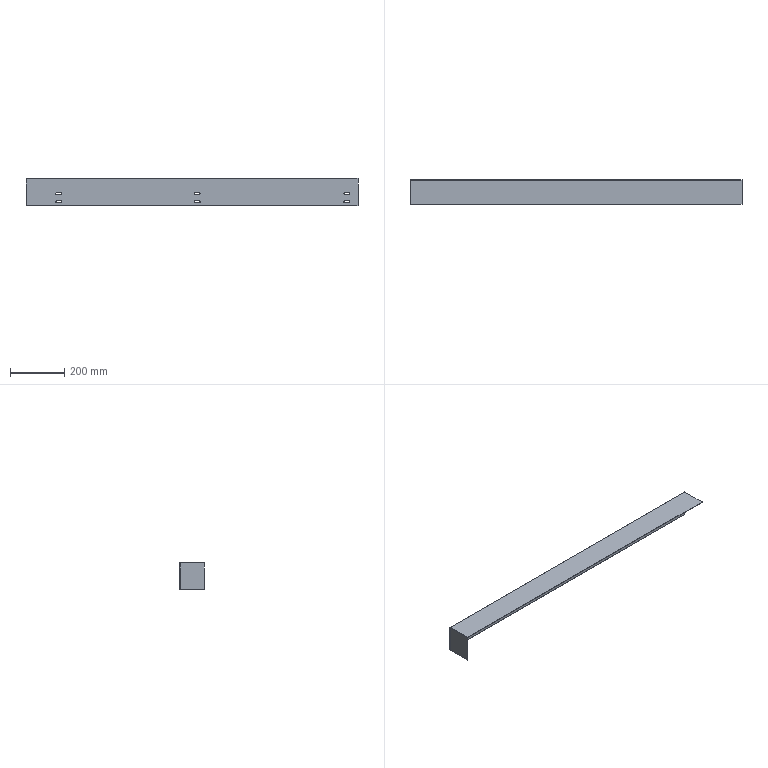Part | SolidWorks | features BaseBody 1 | 1 solid | 41 faces | box 1222 x 91.5 x 101.5 mm | volume 361742 mm3 | plane 25 | cylinder 16 | commonest cylinder face diameters 6 x12 1.473 x2 4.473 x2
STEP:
#1=CARTESIAN_POINT('',(561.,0.,48.));
#2=VERTEX_POINT('',#1);
#3=CARTESIAN_POINT('',(561.,1.5,48.));
#4=VERTEX_POINT('',#3);
#5=CARTESIAN_POINT('',(561.,-90.001,48.));
#6=DIRECTION('',(0.,1.,0.));
#7=VECTOR('',#6,1000.);
#8=LINE('',#5,#7);
#9=EDGE_CURVE('',#2,#4,#8,.T.);
#10=ORIENTED_EDGE('',*,*,#9,.T.);
#11=CARTESIAN_POINT('',(576.,1.5,48.));
#12=VERTEX_POINT('',#11);
#13=CARTESIAN_POINT('',(561.,1.5,48.));
#14=DIRECTION('',(1.,0.,0.));
#15=VECTOR('',#14,1000.);
#16=LINE('',#13,#15);
#17=EDGE_CURVE('',#4,#12,#16,.T.);
#18=ORIENTED_EDGE('',*,*,#17,.T.);
#19=CARTESIAN_POINT('',(576.,0.,48.));
#20=VERTEX_POINT('',#19);
#21=CARTESIAN_POINT('',(576.,-90.001,48.));
#22=DIRECTION('',(0.,1.,0.));
#23=VECTOR('',#22,1000.);
#24=LINE('',#21,#23);
#25=EDGE_CURVE('',#20,#12,#24,.T.);
#26=ORIENTED_EDGE('',*,*,#25,.F.);
#27=CARTESIAN_POINT('',(561.,0.,48.));
#28=DIRECTION('',(1.,0.,0.));
#29=VECTOR('',#28,1000.);
#30=LINE('',#27,#29);
#31=EDGE_CURVE('',#2,#20,#30,.T.);
#32=ORIENTED_EDGE('',*,*,#31,.F.);
#33=EDGE_LOOP('',(#10,#18,#26,#32));
#34=FACE_OUTER_BOUND('',#33,.T.);
#35=CARTESIAN_POINT('',(561.,-90.001,48.));
#36=DIRECTION('',(0.,0.,1.));
#37=DIRECTION('',(0.,-1.,0.));
#38=AXIS2_PLACEMENT_3D('',#35,#36,#37);
#39=PLANE('',#38);
#40=ADVANCED_FACE('',(#34),#39,.F.);
#41=ORIENTED_EDGE('',*,*,#25,.T.);
#42=CARTESIAN_POINT('',(576.,1.5,42.));
#43=VERTEX_POINT('',#42);
#44=CARTESIAN_POINT('',(576.,1.5,45.));
#45=DIRECTION('',(0.,1.,0.));
#46=DIRECTION('',(0.,0.,1.));
#47=AXIS2_PLACEMENT_3D('',#44,#45,#46);
#48=CIRCLE('',#47,3.);
#49=EDGE_CURVE('',#12,#43,#48,.T.);
#50=ORIENTED_EDGE('',*,*,#49,.T.);
#51=CARTESIAN_POINT('',(576.,0.,42.));
#52=VERTEX_POINT('',#51);
#53=CARTESIAN_POINT('',(576.,-90.001,42.));
#54=DIRECTION('',(0.,1.,0.));
#55=VECTOR('',#54,1000.);
#56=LINE('',#53,#55);
#57=EDGE_CURVE('',#52,#43,#56,.T.);
#58=ORIENTED_EDGE('',*,*,#57,.F.);
#59=CARTESIAN_POINT('',(576.,0.,45.));
#60=DIRECTION('',(0.,1.,0.));
#61=DIRECTION('',(0.,0.,-1.));
#62=AXIS2_PLACEMENT_3D('',#59,#60,#61);
#63=CIRCLE('',#62,3.);
#64=EDGE_CURVE('',#20,#52,#63,.T.);
#65=ORIENTED_EDGE('',*,*,#64,.F.);
#66=EDGE_LOOP('',(#41,#50,#58,#65));
#67=FACE_OUTER_BOUND('',#66,.T.);
#68=CARTESIAN_POINT('',(576.,-90.001,45.));
#69=DIRECTION('',(0.,1.,0.));
#70=DIRECTION('',(0.,0.,1.));
#71=AXIS2_PLACEMENT_3D('',#68,#69,#70);
#72=CYLINDRICAL_SURFACE('',#71,3.);
#73=ADVANCED_FACE('',(#67),#72,.F.);
#74=ORIENTED_EDGE('',*,*,#57,.T.);
#75=CARTESIAN_POINT('',(561.,1.5,42.));
#76=VERTEX_POINT('',#75);
#77=CARTESIAN_POINT('',(561.,1.5,42.));
#78=DIRECTION('',(-1.,0.,0.));
#79=VECTOR('',#78,1000.);
#80=LINE('',#77,#79);
#81=EDGE_CURVE('',#43,#76,#80,.T.);
#82=ORIENTED_EDGE('',*,*,#81,.T.);
#83=CARTESIAN_POINT('',(561.,0.,42.));
#84=VERTEX_POINT('',#83);
#85=CARTESIAN_POINT('',(561.,-90.001,42.));
#86=DIRECTION('',(0.,1.,0.));
#87=VECTOR('',#86,1000.);
#88=LINE('',#85,#87);
#89=EDGE_CURVE('',#84,#76,#88,.T.);
#90=ORIENTED_EDGE('',*,*,#89,.F.);
#91=CARTESIAN_POINT('',(561.,0.,42.));
#92=DIRECTION('',(-1.,0.,0.));
#93=VECTOR('',#92,1000.);
#94=LINE('',#91,#93);
#95=EDGE_CURVE('',#52,#84,#94,.T.);
#96=ORIENTED_EDGE('',*,*,#95,.F.);
#97=EDGE_LOOP('',(#74,#82,#90,#96));
#98=FACE_OUTER_BOUND('',#97,.T.);
#99=CARTESIAN_POINT('',(561.,-90.001,42.));
#100=DIRECTION('',(0.,0.,-1.));
#101=DIRECTION('',(-1.,0.,0.));
#102=AXIS2_PLACEMENT_3D('',#99,#100,#101);
#103=PLANE('',#102);
#104=ADVANCED_FACE('',(#98),#103,.F.);
#105=ORIENTED_EDGE('',*,*,#89,.T.);
#106=CARTESIAN_POINT('',(561.,1.5,45.));
#107=DIRECTION('',(0.,1.,0.));
#108=DIRECTION('',(0.,0.,1.));
#109=AXIS2_PLACEMENT_3D('',#106,#107,#108);
#110=CIRCLE('',#109,3.);
#111=EDGE_CURVE('',#76,#4,#110,.T.);
#112=ORIENTED_EDGE('',*,*,#111,.T.);
#113=ORIENTED_EDGE('',*,*,#9,.F.);
#114=CARTESIAN_POINT('',(561.,0.,45.));
#115=DIRECTION('',(0.,1.,0.));
#116=DIRECTION('',(0.,0.,-1.));
#117=AXIS2_PLACEMENT_3D('',#114,#115,#116);
#118=CIRCLE('',#117,3.);
#119=EDGE_CURVE('',#84,#2,#118,.T.);
#120=ORIENTED_EDGE('',*,*,#119,.F.);
#121=EDGE_LOOP('',(#105,#112,#113,#120));
#122=FACE_OUTER_BOUND('',#121,.T.);
#123=CARTESIAN_POINT('',(561.,-90.001,45.));
#124=DIRECTION('',(0.,1.,0.));
#125=DIRECTION('',(0.,0.,1.));
#126=AXIS2_PLACEMENT_3D('',#123,#124,#125);
#127=CYLINDRICAL_SURFACE('',#126,3.);
#128=ADVANCED_FACE('',(#122),#127,.F.);
#129=CARTESIAN_POINT('',(561.,0.,18.));
#130=VERTEX_POINT('',#129);
#131=CARTESIAN_POINT('',(561.,1.5,18.));
#132=VERTEX_POINT('',#131);
#133=CARTESIAN_POINT('',(561.,-90.001,18.));
#134=DIRECTION('',(0.,1.,0.));
#135=VECTOR('',#134,1000.);
#136=LINE('',#133,#135);
#137=EDGE_CURVE('',#130,#132,#136,.T.);
#138=ORIENTED_EDGE('',*,*,#137,.T.);
#139=CARTESIAN_POINT('',(576.,1.5,18.));
#140=VERTEX_POINT('',#139);
#141=CARTESIAN_POINT('',(561.,1.5,18.));
#142=DIRECTION('',(1.,0.,0.));
#143=VECTOR('',#142,1000.);
#144=LINE('',#141,#143);
#145=EDGE_CURVE('',#132,#140,#144,.T.);
#146=ORIENTED_EDGE('',*,*,#145,.T.);
#147=CARTESIAN_POINT('',(576.,0.,18.));
#148=VERTEX_POINT('',#147);
#149=CARTESIAN_POINT('',(576.,-90.001,18.));
#150=DIRECTION('',(0.,1.,0.));
#151=VECTOR('',#150,1000.);
#152=LINE('',#149,#151);
#153=EDGE_CURVE('',#148,#140,#152,.T.);
#154=ORIENTED_EDGE('',*,*,#153,.F.);
#155=CARTESIAN_POINT('',(561.,0.,18.));
#156=DIRECTION('',(1.,0.,0.));
#157=VECTOR('',#156,1000.);
#158=LINE('',#155,#157);
#159=EDGE_CURVE('',#130,#148,#158,.T.);
#160=ORIENTED_EDGE('',*,*,#159,.F.);
#161=EDGE_LOOP('',(#138,#146,#154,#160));
#162=FACE_OUTER_BOUND('',#161,.T.);
#163=CARTESIAN_POINT('',(561.,-90.001,18.));
#164=DIRECTION('',(0.,0.,1.));
#165=DIRECTION('',(0.,-1.,0.));
#166=AXIS2_PLACEMENT_3D('',#163,#164,#165);
#167=PLANE('',#166);
#168=ADVANCED_FACE('',(#162),#167,.F.);
#169=ORIENTED_EDGE('',*,*,#153,.T.);
#170=CARTESIAN_POINT('',(576.,1.5,12.));
#171=VERTEX_POINT('',#170);
#172=CARTESIAN_POINT('',(576.,1.5,15.));
#173=DIRECTION('',(0.,1.,0.));
#174=DIRECTION('',(0.,0.,1.));
#175=AXIS2_PLACEMENT_3D('',#172,#173,#174);
#176=CIRCLE('',#175,3.);
#177=EDGE_CURVE('',#140,#171,#176,.T.);
#178=ORIENTED_EDGE('',*,*,#177,.T.);
#179=CARTESIAN_POINT('',(576.,0.,12.));
#180=VERTEX_POINT('',#179);
#181=CARTESIAN_POINT('',(576.,-90.001,12.));
#182=DIRECTION('',(0.,1.,0.));
#183=VECTOR('',#182,1000.);
#184=LINE('',#181,#183);
#185=EDGE_CURVE('',#180,#171,#184,.T.);
#186=ORIENTED_EDGE('',*,*,#185,.F.);
#187=CARTESIAN_POINT('',(576.,0.,15.));
#188=DIRECTION('',(0.,1.,0.));
#189=DIRECTION('',(0.,0.,-1.));
#190=AXIS2_PLACEMENT_3D('',#187,#188,#189);
#191=CIRCLE('',#190,3.);
#192=EDGE_CURVE('',#148,#180,#191,.T.);
#193=ORIENTED_EDGE('',*,*,#192,.F.);
#194=EDGE_LOOP('',(#169,#178,#186,#193));
#195=FACE_OUTER_BOUND('',#194,.T.);
#196=CARTESIAN_POINT('',(576.,-90.001,15.));
#197=DIRECTION('',(0.,1.,0.));
#198=DIRECTION('',(0.,0.,1.));
#199=AXIS2_PLACEMENT_3D('',#196,#197,#198);
#200=CYLINDRICAL_SURFACE('',#199,3.);
#201=ADVANCED_FACE('',(#195),#200,.F.);
#202=ORIENTED_EDGE('',*,*,#185,.T.);
#203=CARTESIAN_POINT('',(561.,1.5,12.));
#204=VERTEX_POINT('',#203);
#205=CARTESIAN_POINT('',(561.,1.5,12.));
#206=DIRECTION('',(-1.,0.,0.));
#207=VECTOR('',#206,1000.);
#208=LINE('',#205,#207);
#209=EDGE_CURVE('',#171,#204,#208,.T.);
#210=ORIENTED_EDGE('',*,*,#209,.T.);
#211=CARTESIAN_POINT('',(561.,0.,12.));
#212=VERTEX_POINT('',#211);
#213=CARTESIAN_POINT('',(561.,-90.001,12.));
#214=DIRECTION('',(0.,1.,0.));
#215=VECTOR('',#214,1000.);
#216=LINE('',#213,#215);
#217=EDGE_CURVE('',#212,#204,#216,.T.);
#218=ORIENTED_EDGE('',*,*,#217,.F.);
#219=CARTESIAN_POINT('',(561.,0.,12.));
#220=DIRECTION('',(-1.,0.,0.));
#221=VECTOR('',#220,1000.);
#222=LINE('',#219,#221);
#223=EDGE_CURVE('',#180,#212,#222,.T.);
#224=ORIENTED_EDGE('',*,*,#223,.F.);
#225=EDGE_LOOP('',(#202,#210,#218,#224));
#226=FACE_OUTER_BOUND('',#225,.T.);
#227=CARTESIAN_POINT('',(561.,-90.001,12.));
#228=DIRECTION('',(0.,0.,-1.));
#229=DIRECTION('',(-1.,0.,0.));
#230=AXIS2_PLACEMENT_3D('',#227,#228,#229);
#231=PLANE('',#230);
#232=ADVANCED_FACE('',(#226),#231,.F.);
#233=ORIENTED_EDGE('',*,*,#217,.T.);
#234=CARTESIAN_POINT('',(561.,1.5,15.));
#235=DIRECTION('',(0.,1.,0.));
#236=DIRECTION('',(0.,0.,1.));
#237=AXIS2_PLACEMENT_3D('',#234,#235,#236);
#238=CIRCLE('',#237,3.);
#239=EDGE_CURVE('',#204,#132,#238,.T.);
#240=ORIENTED_EDGE('',*,*,#239,.T.);
#241=ORIENTED_EDGE('',*,*,#137,.F.);
#242=CARTESIAN_POINT('',(561.,0.,15.));
#243=DIRECTION('',(0.,1.,0.));
#244=DIRECTION('',(0.,0.,-1.));
#245=AXIS2_PLACEMENT_3D('',#242,#243,#244);
#246=CIRCLE('',#245,3.);
#247=EDGE_CURVE('',#212,#130,#246,.T.);
#248=ORIENTED_EDGE('',*,*,#247,.F.);
#249=EDGE_LOOP('',(#233,#240,#241,#248));
#250=FACE_OUTER_BOUND('',#249,.T.);
#251=CARTESIAN_POINT('',(561.,-90.001,15.));
#252=DIRECTION('',(0.,1.,0.));
#253=DIRECTION('',(0.,0.,1.));
#254=AXIS2_PLACEMENT_3D('',#251,#252,#253);
#255=CYLINDRICAL_SURFACE('',#254,3.);
#256=ADVANCED_FACE('',(#250),#255,.F.);
#257=CARTESIAN_POINT('',(26.,0.,12.));
#258=VERTEX_POINT('',#257);
#259=CARTESIAN_POINT('',(26.,1.5,12.));
#260=VERTEX_POINT('',#259);
#261=CARTESIAN_POINT('',(26.,-90.001,12.));
#262=DIRECTION('',(0.,1.,0.));
#263=VECTOR('',#262,1000.);
#264=LINE('',#261,#263);
#265=EDGE_CURVE('',#258,#260,#264,.T.);
#266=ORIENTED_EDGE('',*,*,#265,.T.);
#267=CARTESIAN_POINT('',(11.,1.5,12.));
#268=VERTEX_POINT('',#267);
#269=CARTESIAN_POINT('',(26.,1.5,12.));
#270=DIRECTION('',(-1.,0.,0.));
#271=VECTOR('',#270,1000.);
#272=LINE('',#269,#271);
#273=EDGE_CURVE('',#260,#268,#272,.T.);
#274=ORIENTED_EDGE('',*,*,#273,.T.);
#275=CARTESIAN_POINT('',(11.,0.,12.));
#276=VERTEX_POINT('',#275);
#277=CARTESIAN_POINT('',(11.,-90.001,12.));
#278=DIRECTION('',(0.,1.,0.));
#279=VECTOR('',#278,1000.);
#280=LINE('',#277,#279);
#281=EDGE_CURVE('',#276,#268,#280,.T.);
#282=ORIENTED_EDGE('',*,*,#281,.F.);
#283=CARTESIAN_POINT('',(26.,0.,12.));
#284=DIRECTION('',(-1.,0.,0.));
#285=VECTOR('',#284,1000.);
#286=LINE('',#283,#285);
#287=EDGE_CURVE('',#258,#276,#286,.T.);
#288=ORIENTED_EDGE('',*,*,#287,.F.);
#289=EDGE_LOOP('',(#266,#274,#282,#288));
#290=FACE_OUTER_BOUND('',#289,.T.);
#291=CARTESIAN_POINT('',(26.,-90.001,12.));
#292=DIRECTION('',(0.,0.,-1.));
#293=DIRECTION('',(-1.,0.,0.));
#294=AXIS2_PLACEMENT_3D('',#291,#292,#293);
#295=PLANE('',#294);
#296=ADVANCED_FACE('',(#290),#295,.F.);
#297=ORIENTED_EDGE('',*,*,#281,.T.);
#298=CARTESIAN_POINT('',(11.,1.5,18.));
#299=VERTEX_POINT('',#298);
#300=CARTESIAN_POINT('',(11.,1.5,15.));
#301=DIRECTION('',(0.,1.,0.));
#302=DIRECTION('',(0.,0.,-1.));
#303=AXIS2_PLACEMENT_3D('',#300,#301,#302);
#304=CIRCLE('',#303,3.);
#305=EDGE_CURVE('',#268,#299,#304,.T.);
#306=ORIENTED_EDGE('',*,*,#305,.T.);
#307=CARTESIAN_POINT('',(11.,0.,18.));
#308=VERTEX_POINT('',#307);
#309=CARTESIAN_POINT('',(11.,-90.001,18.));
#310=DIRECTION('',(0.,1.,0.));
#311=VECTOR('',#310,1000.);
#312=LINE('',#309,#311);
#313=EDGE_CURVE('',#308,#299,#312,.T.);
#314=ORIENTED_EDGE('',*,*,#313,.F.);
#315=CARTESIAN_POINT('',(11.,0.,15.));
#316=DIRECTION('',(0.,1.,0.));
#317=DIRECTION('',(0.,0.,-1.));
#318=AXIS2_PLACEMENT_3D('',#315,#316,#317);
#319=CIRCLE('',#318,3.);
#320=EDGE_CURVE('',#276,#308,#319,.T.);
#321=ORIENTED_EDGE('',*,*,#320,.F.);
#322=EDGE_LOOP('',(#297,#306,#314,#321));
#323=FACE_OUTER_BOUND('',#322,.T.);
#324=CARTESIAN_POINT('',(11.,-90.001,15.));
#325=DIRECTION('',(0.,1.,0.));
#326=DIRECTION('',(0.,0.,1.));
#327=AXIS2_PLACEMENT_3D('',#324,#325,#326);
#328=CYLINDRICAL_SURFACE('',#327,3.);
#329=ADVANCED_FACE('',(#323),#328,.F.);
#330=ORIENTED_EDGE('',*,*,#313,.T.);
#331=CARTESIAN_POINT('',(26.,1.5,18.));
#332=VERTEX_POINT('',#331);
#333=CARTESIAN_POINT('',(26.,1.5,18.));
#334=DIRECTION('',(1.,0.,0.));
#335=VECTOR('',#334,1000.);
#336=LINE('',#333,#335);
#337=EDGE_CURVE('',#299,#332,#336,.T.);
#338=ORIENTED_EDGE('',*,*,#337,.T.);
#339=CARTESIAN_POINT('',(26.,0.,18.));
#340=VERTEX_POINT('',#339);
#341=CARTESIAN_POINT('',(26.,-90.001,18.));
#342=DIRECTION('',(0.,1.,0.));
#343=VECTOR('',#342,1000.);
#344=LINE('',#341,#343);
#345=EDGE_CURVE('',#340,#332,#344,.T.);
#346=ORIENTED_EDGE('',*,*,#345,.F.);
#347=CARTESIAN_POINT('',(26.,0.,18.));
#348=DIRECTION('',(1.,0.,0.));
#349=VECTOR('',#348,1000.);
#350=LINE('',#347,#349);
#351=EDGE_CURVE('',#308,#340,#350,.T.);
#352=ORIENTED_EDGE('',*,*,#351,.F.);
#353=EDGE_LOOP('',(#330,#338,#346,#352));
#354=FACE_OUTER_BOUND('',#353,.T.);
#355=CARTESIAN_POINT('',(26.,-90.001,18.));
#356=DIRECTION('',(0.,0.,1.));
#357=DIRECTION('',(0.,-1.,0.));
#358=AXIS2_PLACEMENT_3D('',#355,#356,#357);
#359=PLANE('',#358);
#360=ADVANCED_FACE('',(#354),#359,.F.);
#361=ORIENTED_EDGE('',*,*,#345,.T.);
#362=CARTESIAN_POINT('',(26.,1.5,15.));
#363=DIRECTION('',(0.,1.,0.));
#364=DIRECTION('',(0.,0.,-1.));
#365=AXIS2_PLACEMENT_3D('',#362,#363,#364);
#366=CIRCLE('',#365,3.);
#367=EDGE_CURVE('',#332,#260,#366,.T.);
#368=ORIENTED_EDGE('',*,*,#367,.T.);
#369=ORIENTED_EDGE('',*,*,#265,.F.);
#370=CARTESIAN_POINT('',(26.,0.,15.));
#371=DIRECTION('',(0.,1.,0.));
#372=DIRECTION('',(0.,0.,-1.));
#373=AXIS2_PLACEMENT_3D('',#370,#371,#372);
#374=CIRCLE('',#373,3.);
#375=EDGE_CURVE('',#340,#258,#374,.T.);
#376=ORIENTED_EDGE('',*,*,#375,.F.);
#377=EDGE_LOOP('',(#361,#368,#369,#376));
#378=FACE_OUTER_BOUND('',#377,.T.);
#379=CARTESIAN_POINT('',(26.,-90.001,15.));
#380=DIRECTION('',(0.,1.,0.));
#381=DIRECTION('',(0.,0.,1.));
#382=AXIS2_PLACEMENT_3D('',#379,#380,#381);
#383=CYLINDRICAL_SURFACE('',#382,3.);
#384=ADVANCED_FACE('',(#378),#383,.F.);
#385=CARTESIAN_POINT('',(26.,0.,42.));
#386=VERTEX_POINT('',#385);
#387=CARTESIAN_POINT('',(26.,1.5,42.));
#388=VERTEX_POINT('',#387);
#389=CARTESIAN_POINT('',(26.,-90.001,42.));
#390=DIRECTION('',(0.,1.,0.));
#391=VECTOR('',#390,1000.);
#392=LINE('',#389,#391);
#393=EDGE_CURVE('',#386,#388,#392,.T.);
#394=ORIENTED_EDGE('',*,*,#393,.T.);
#395=CARTESIAN_POINT('',(11.,1.5,42.));
#396=VERTEX_POINT('',#395);
#397=CARTESIAN_POINT('',(26.,1.5,42.));
#398=DIRECTION('',(-1.,0.,0.));
#399=VECTOR('',#398,1000.);
#400=LINE('',#397,#399);
#401=EDGE_CURVE('',#388,#396,#400,.T.);
#402=ORIENTED_EDGE('',*,*,#401,.T.);
#403=CARTESIAN_POINT('',(11.,0.,42.));
#404=VERTEX_POINT('',#403);
#405=CARTESIAN_POINT('',(11.,-90.001,42.));
#406=DIRECTION('',(0.,1.,0.));
#407=VECTOR('',#406,1000.);
#408=LINE('',#405,#407);
#409=EDGE_CURVE('',#404,#396,#408,.T.);
#410=ORIENTED_EDGE('',*,*,#409,.F.);
#411=CARTESIAN_POINT('',(26.,0.,42.));
#412=DIRECTION('',(-1.,0.,0.));
#413=VECTOR('',#412,1000.);
#414=LINE('',#411,#413);
#415=EDGE_CURVE('',#386,#404,#414,.T.);
#416=ORIENTED_EDGE('',*,*,#415,.F.);
#417=EDGE_LOOP('',(#394,#402,#410,#416));
#418=FACE_OUTER_BOUND('',#417,.T.);
#419=CARTESIAN_POINT('',(26.,-90.001,42.));
#420=DIRECTION('',(0.,0.,-1.));
#421=DIRECTION('',(-1.,0.,0.));
#422=AXIS2_PLACEMENT_3D('',#419,#420,#421);
#423=PLANE('',#422);
#424=ADVANCED_FACE('',(#418),#423,.F.);
#425=ORIENTED_EDGE('',*,*,#409,.T.);
#426=CARTESIAN_POINT('',(11.,1.5,48.));
#427=VERTEX_POINT('',#426);
#428=CARTESIAN_POINT('',(11.,1.5,45.));
#429=DIRECTION('',(0.,1.,0.));
#430=DIRECTION('',(0.,0.,-1.));
#431=AXIS2_PLACEMENT_3D('',#428,#429,#430);
#432=CIRCLE('',#431,3.);
#433=EDGE_CURVE('',#396,#427,#432,.T.);
#434=ORIENTED_EDGE('',*,*,#433,.T.);
#435=CARTESIAN_POINT('',(11.,0.,48.));
#436=VERTEX_POINT('',#435);
#437=CARTESIAN_POINT('',(11.,-90.001,48.));
#438=DIRECTION('',(0.,1.,0.));
#439=VECTOR('',#438,1000.);
#440=LINE('',#437,#439);
#441=EDGE_CURVE('',#436,#427,#440,.T.);
#442=ORIENTED_EDGE('',*,*,#441,.F.);
#443=CARTESIAN_POINT('',(11.,0.,45.));
#444=DIRECTION('',(0.,1.,0.));
#445=DIRECTION('',(0.,0.,-1.));
#446=AXIS2_PLACEMENT_3D('',#443,#444,#445);
#447=CIRCLE('',#446,3.);
#448=EDGE_CURVE('',#404,#436,#447,.T.);
#449=ORIENTED_EDGE('',*,*,#448,.F.);
#450=EDGE_LOOP('',(#425,#434,#442,#449));
#451=FACE_OUTER_BOUND('',#450,.T.);
#452=CARTESIAN_POINT('',(11.,-90.001,45.));
#453=DIRECTION('',(0.,1.,0.));
#454=DIRECTION('',(0.,0.,1.));
#455=AXIS2_PLACEMENT_3D('',#452,#453,#454);
#456=CYLINDRICAL_SURFACE('',#455,3.);
#457=ADVANCED_FACE('',(#451),#456,.F.);
#458=ORIENTED_EDGE('',*,*,#441,.T.);
#459=CARTESIAN_POINT('',(26.,1.5,48.));
#460=VERTEX_POINT('',#459);
#461=CARTESIAN_POINT('',(26.,1.5,48.));
#462=DIRECTION('',(1.,0.,0.));
#463=VECTOR('',#462,1000.);
#464=LINE('',#461,#463);
#465=EDGE_CURVE('',#427,#460,#464,.T.);
#466=ORIENTED_EDGE('',*,*,#465,.T.);
#467=CARTESIAN_POINT('',(26.,0.,48.));
#468=VERTEX_POINT('',#467);
#469=CARTESIAN_POINT('',(26.,-90.001,48.));
#470=DIRECTION('',(0.,1.,0.));
#471=VECTOR('',#470,1000.);
#472=LINE('',#469,#471);
#473=EDGE_CURVE('',#468,#460,#472,.T.);
#474=ORIENTED_EDGE('',*,*,#473,.F.);
#475=CARTESIAN_POINT('',(26.,0.,48.));
#476=DIRECTION('',(1.,0.,0.));
#477=VECTOR('',#476,1000.);
#478=LINE('',#475,#477);
#479=EDGE_CURVE('',#436,#468,#478,.T.);
#480=ORIENTED_EDGE('',*,*,#479,.F.);
#481=EDGE_LOOP('',(#458,#466,#474,#480));
#482=FACE_OUTER_BOUND('',#481,.T.);
#483=CARTESIAN_POINT('',(26.,-90.001,48.));
#484=DIRECTION('',(0.,0.,1.));
#485=DIRECTION('',(0.,-1.,0.));
#486=AXIS2_PLACEMENT_3D('',#483,#484,#485);
#487=PLANE('',#486);
#488=ADVANCED_FACE('',(#482),#487,.F.);
#489=ORIENTED_EDGE('',*,*,#473,.T.);
#490=CARTESIAN_POINT('',(26.,1.5,45.));
#491=DIRECTION('',(0.,1.,0.));
#492=DIRECTION('',(0.,0.,-1.));
#493=AXIS2_PLACEMENT_3D('',#490,#491,#492);
#494=CIRCLE('',#493,3.);
#495=EDGE_CURVE('',#460,#388,#494,.T.);
#496=ORIENTED_EDGE('',*,*,#495,.T.);
#497=ORIENTED_EDGE('',*,*,#393,.F.);
#498=CARTESIAN_POINT('',(26.,0.,45.));
#499=DIRECTION('',(0.,1.,0.));
#500=DIRECTION('',(0.,0.,-1.));
#501=AXIS2_PLACEMENT_3D('',#498,#499,#500);
#502=CIRCLE('',#501,3.);
#503=EDGE_CURVE('',#468,#386,#502,.T.);
#504=ORIENTED_EDGE('',*,*,#503,.F.);
#505=EDGE_LOOP('',(#489,#496,#497,#504));
#506=FACE_OUTER_BOUND('',#505,.T.);
#507=CARTESIAN_POINT('',(26.,-90.001,45.));
#508=DIRECTION('',(0.,1.,0.));
#509=DIRECTION('',(0.,0.,1.));
#510=AXIS2_PLACEMENT_3D('',#507,#508,#509);
#511=CYLINDRICAL_SURFACE('',#510,3.);
#512=ADVANCED_FACE('',(#506),#511,.F.);
#513=CARTESIAN_POINT('',(-499.,0.,48.));
#514=VERTEX_POINT('',#513);
#515=CARTESIAN_POINT('',(-499.,1.5,48.));
#516=VERTEX_POINT('',#515);
#517=CARTESIAN_POINT('',(-499.,-90.001,48.));
#518=DIRECTION('',(0.,1.,0.));
#519=VECTOR('',#518,1000.);
#520=LINE('',#517,#519);
#521=EDGE_CURVE('',#514,#516,#520,.T.);
#522=ORIENTED_EDGE('',*,*,#521,.T.);
#523=CARTESIAN_POINT('',(-484.,1.5,48.));
#524=VERTEX_POINT('',#523);
#525=CARTESIAN_POINT('',(-499.,1.5,48.));
#526=DIRECTION('',(1.,0.,0.));
#527=VECTOR('',#526,1000.);
#528=LINE('',#525,#527);
#529=EDGE_CURVE('',#516,#524,#528,.T.);
#530=ORIENTED_EDGE('',*,*,#529,.T.);
#531=CARTESIAN_POINT('',(-484.,0.,48.));
#532=VERTEX_POINT('',#531);
#533=CARTESIAN_POINT('',(-484.,-90.001,48.));
#534=DIRECTION('',(0.,1.,0.));
#535=VECTOR('',#534,1000.);
#536=LINE('',#533,#535);
#537=EDGE_CURVE('',#532,#524,#536,.T.);
#538=ORIENTED_EDGE('',*,*,#537,.F.);
#539=CARTESIAN_POINT('',(-499.,0.,48.));
#540=DIRECTION('',(1.,0.,0.));
#541=VECTOR('',#540,1000.);
#542=LINE('',#539,#541);
#543=EDGE_CURVE('',#514,#532,#542,.T.);
#544=ORIENTED_EDGE('',*,*,#543,.F.);
#545=EDGE_LOOP('',(#522,#530,#538,#544));
#546=FACE_OUTER_BOUND('',#545,.T.);
#547=CARTESIAN_POINT('',(-499.,-90.001,48.));
#548=DIRECTION('',(0.,0.,1.));
#549=DIRECTION('',(0.,-1.,0.));
#550=AXIS2_PLACEMENT_3D('',#547,#548,#549);
#551=PLANE('',#550);
#552=ADVANCED_FACE('',(#546),#551,.F.);
#553=ORIENTED_EDGE('',*,*,#537,.T.);
#554=CARTESIAN_POINT('',(-484.,1.5,42.));
#555=VERTEX_POINT('',#554);
#556=CARTESIAN_POINT('',(-484.,1.5,45.));
#557=DIRECTION('',(0.,1.,0.));
#558=DIRECTION('',(0.,0.,1.));
#559=AXIS2_PLACEMENT_3D('',#556,#557,#558);
#560=CIRCLE('',#559,3.);
#561=EDGE_CURVE('',#524,#555,#560,.T.);
#562=ORIENTED_EDGE('',*,*,#561,.T.);
#563=CARTESIAN_POINT('',(-484.,0.,42.));
#564=VERTEX_POINT('',#563);
#565=CARTESIAN_POINT('',(-484.,-90.001,42.));
#566=DIRECTION('',(0.,1.,0.));
#567=VECTOR('',#566,1000.);
#568=LINE('',#565,#567);
#569=EDGE_CURVE('',#564,#555,#568,.T.);
#570=ORIENTED_EDGE('',*,*,#569,.F.);
#571=CARTESIAN_POINT('',(-484.,0.,45.));
#572=DIRECTION('',(0.,1.,0.));
#573=DIRECTION('',(0.,0.,-1.));
#574=AXIS2_PLACEMENT_3D('',#571,#572,#573);
#575=CIRCLE('',#574,3.);
#576=EDGE_CURVE('',#532,#564,#575,.T.);
#577=ORIENTED_EDGE('',*,*,#576,.F.);
#578=EDGE_LOOP('',(#553,#562,#570,#577));
#579=FACE_OUTER_BOUND('',#578,.T.);
#580=CARTESIAN_POINT('',(-484.,-90.001,45.));
#581=DIRECTION('',(0.,1.,0.));
#582=DIRECTION('',(0.,0.,1.));
#583=AXIS2_PLACEMENT_3D('',#580,#581,#582);
#584=CYLINDRICAL_SURFACE('',#583,3.);
#585=ADVANCED_FACE('',(#579),#584,.F.);
#586=ORIENTED_EDGE('',*,*,#569,.T.);
#587=CARTESIAN_POINT('',(-499.,1.5,42.));
#588=VERTEX_POINT('',#587);
#589=CARTESIAN_POINT('',(-499.,1.5,42.));
#590=DIRECTION('',(-1.,0.,0.));
#591=VECTOR('',#590,1000.);
#592=LINE('',#589,#591);
#593=EDGE_CURVE('',#555,#588,#592,.T.);
#594=ORIENTED_EDGE('',*,*,#593,.T.);
#595=CARTESIAN_POINT('',(-499.,0.,42.));
#596=VERTEX_POINT('',#595);
#597=CARTESIAN_POINT('',(-499.,-90.001,42.));
#598=DIRECTION('',(0.,1.,0.));
#599=VECTOR('',#598,1000.);
#600=LINE('',#597,#599);
#601=EDGE_CURVE('',#596,#588,#600,.T.);
#602=ORIENTED_EDGE('',*,*,#601,.F.);
#603=CARTESIAN_POINT('',(-499.,0.,42.));
#604=DIRECTION('',(-1.,0.,0.));
#605=VECTOR('',#604,1000.);
#606=LINE('',#603,#605);
#607=EDGE_CURVE('',#564,#596,#606,.T.);
#608=ORIENTED_EDGE('',*,*,#607,.F.);
#609=EDGE_LOOP('',(#586,#594,#602,#608));
#610=FACE_OUTER_BOUND('',#609,.T.);
#611=CARTESIAN_POINT('',(-499.,-90.001,42.));
#612=DIRECTION('',(0.,0.,-1.));
#613=DIRECTION('',(-1.,0.,0.));
#614=AXIS2_PLACEMENT_3D('',#611,#612,#613);
#615=PLANE('',#614);
#616=ADVANCED_FACE('',(#610),#615,.F.);
#617=ORIENTED_EDGE('',*,*,#601,.T.);
#618=CARTESIAN_POINT('',(-499.,1.5,45.));
#619=DIRECTION('',(0.,1.,0.));
#620=DIRECTION('',(0.,0.,1.));
#621=AXIS2_PLACEMENT_3D('',#618,#619,#620);
#622=CIRCLE('',#621,3.);
#623=EDGE_CURVE('',#588,#516,#622,.T.);
#624=ORIENTED_EDGE('',*,*,#623,.T.);
#625=ORIENTED_EDGE('',*,*,#521,.F.);
#626=CARTESIAN_POINT('',(-499.,0.,45.));
#627=DIRECTION('',(0.,1.,0.));
#628=DIRECTION('',(0.,0.,-1.));
#629=AXIS2_PLACEMENT_3D('',#626,#627,#628);
#630=CIRCLE('',#629,3.);
#631=EDGE_CURVE('',#596,#514,#630,.T.);
#632=ORIENTED_EDGE('',*,*,#631,.F.);
#633=EDGE_LOOP('',(#617,#624,#625,#632));
#634=FACE_OUTER_BOUND('',#633,.T.);
#635=CARTESIAN_POINT('',(-499.,-90.001,45.));
#636=DIRECTION('',(0.,1.,0.));
#637=DIRECTION('',(0.,0.,1.));
#638=AXIS2_PLACEMENT_3D('',#635,#636,#637);
#639=CYLINDRICAL_SURFACE('',#638,3.);
#640=ADVANCED_FACE('',(#634),#639,.F.);
#641=CARTESIAN_POINT('',(-499.,0.,18.));
#642=VERTEX_POINT('',#641);
#643=CARTESIAN_POINT('',(-499.,1.5,18.));
#644=VERTEX_POINT('',#643);
#645=CARTESIAN_POINT('',(-499.,-90.001,18.));
#646=DIRECTION('',(0.,1.,0.));
#647=VECTOR('',#646,1000.);
#648=LINE('',#645,#647);
#649=EDGE_CURVE('',#642,#644,#648,.T.);
#650=ORIENTED_EDGE('',*,*,#649,.T.);
#651=CARTESIAN_POINT('',(-484.,1.5,18.));
#652=VERTEX_POINT('',#651);
#653=CARTESIAN_POINT('',(-499.,1.5,18.));
#654=DIRECTION('',(1.,0.,0.));
#655=VECTOR('',#654,1000.);
#656=LINE('',#653,#655);
#657=EDGE_CURVE('',#644,#652,#656,.T.);
#658=ORIENTED_EDGE('',*,*,#657,.T.);
#659=CARTESIAN_POINT('',(-484.,0.,18.));
#660=VERTEX_POINT('',#659);
#661=CARTESIAN_POINT('',(-484.,-90.001,18.));
#662=DIRECTION('',(0.,1.,0.));
#663=VECTOR('',#662,1000.);
#664=LINE('',#661,#663);
#665=EDGE_CURVE('',#660,#652,#664,.T.);
#666=ORIENTED_EDGE('',*,*,#665,.F.);
#667=CARTESIAN_POINT('',(-499.,0.,18.));
#668=DIRECTION('',(1.,0.,0.));
#669=VECTOR('',#668,1000.);
#670=LINE('',#667,#669);
#671=EDGE_CURVE('',#642,#660,#670,.T.);
#672=ORIENTED_EDGE('',*,*,#671,.F.);
#673=EDGE_LOOP('',(#650,#658,#666,#672));
#674=FACE_OUTER_BOUND('',#673,.T.);
#675=CARTESIAN_POINT('',(-499.,-90.001,18.));
#676=DIRECTION('',(0.,0.,1.));
#677=DIRECTION('',(1.,0.,0.));
#678=AXIS2_PLACEMENT_3D('',#675,#676,#677);
#679=PLANE('',#678);
#680=ADVANCED_FACE('',(#674),#679,.F.);
#681=ORIENTED_EDGE('',*,*,#665,.T.);
#682=CARTESIAN_POINT('',(-484.,1.5,12.));
#683=VERTEX_POINT('',#682);
#684=CARTESIAN_POINT('',(-484.,1.5,15.));
#685=DIRECTION('',(0.,1.,0.));
#686=DIRECTION('',(0.,0.,1.));
#687=AXIS2_PLACEMENT_3D('',#684,#685,#686);
#688=CIRCLE('',#687,3.);
#689=EDGE_CURVE('',#652,#683,#688,.T.);
#690=ORIENTED_EDGE('',*,*,#689,.T.);
#691=CARTESIAN_POINT('',(-484.,0.,12.));
#692=VERTEX_POINT('',#691);
#693=CARTESIAN_POINT('',(-484.,-90.001,12.));
#694=DIRECTION('',(0.,1.,0.));
#695=VECTOR('',#694,1000.);
#696=LINE('',#693,#695);
#697=EDGE_CURVE('',#692,#683,#696,.T.);
#698=ORIENTED_EDGE('',*,*,#697,.F.);
#699=CARTESIAN_POINT('',(-484.,0.,15.));
#700=DIRECTION('',(0.,1.,0.));
#701=DIRECTION('',(0.,0.,-1.));
#702=AXIS2_PLACEMENT_3D('',#699,#700,#701);
#703=CIRCLE('',#702,3.);
#704=EDGE_CURVE('',#660,#692,#703,.T.);
#705=ORIENTED_EDGE('',*,*,#704,.F.);
#706=EDGE_LOOP('',(#681,#690,#698,#705));
#707=FACE_OUTER_BOUND('',#706,.T.);
#708=CARTESIAN_POINT('',(-484.,-90.001,15.));
#709=DIRECTION('',(0.,1.,0.));
#710=DIRECTION('',(0.,0.,1.));
#711=AXIS2_PLACEMENT_3D('',#708,#709,#710);
#712=CYLINDRICAL_SURFACE('',#711,3.);
#713=ADVANCED_FACE('',(#707),#712,.F.);
#714=ORIENTED_EDGE('',*,*,#697,.T.);
#715=CARTESIAN_POINT('',(-499.,1.5,12.));
#716=VERTEX_POINT('',#715);
#717=CARTESIAN_POINT('',(-499.,1.5,12.));
#718=DIRECTION('',(-1.,0.,0.));
#719=VECTOR('',#718,1000.);
#720=LINE('',#717,#719);
#721=EDGE_CURVE('',#683,#716,#720,.T.);
#722=ORIENTED_EDGE('',*,*,#721,.T.);
#723=CARTESIAN_POINT('',(-499.,0.,12.));
#724=VERTEX_POINT('',#723);
#725=CARTESIAN_POINT('',(-499.,-90.001,12.));
#726=DIRECTION('',(0.,1.,0.));
#727=VECTOR('',#726,1000.);
#728=LINE('',#725,#727);
#729=EDGE_CURVE('',#724,#716,#728,.T.);
#730=ORIENTED_EDGE('',*,*,#729,.F.);
#731=CARTESIAN_POINT('',(-499.,0.,12.));
#732=DIRECTION('',(-1.,0.,0.));
#733=VECTOR('',#732,1000.);
#734=LINE('',#731,#733);
#735=EDGE_CURVE('',#692,#724,#734,.T.);
#736=ORIENTED_EDGE('',*,*,#735,.F.);
#737=EDGE_LOOP('',(#714,#722,#730,#736));
#738=FACE_OUTER_BOUND('',#737,.T.);
#739=CARTESIAN_POINT('',(-499.,-90.001,12.));
#740=DIRECTION('',(0.,0.,-1.));
#741=DIRECTION('',(-1.,0.,0.));
#742=AXIS2_PLACEMENT_3D('',#739,#740,#741);
#743=PLANE('',#742);
#744=ADVANCED_FACE('',(#738),#743,.F.);
#745=ORIENTED_EDGE('',*,*,#729,.T.);
#746=CARTESIAN_POINT('',(-499.,1.5,15.));
#747=DIRECTION('',(0.,1.,0.));
#748=DIRECTION('',(0.,0.,1.));
#749=AXIS2_PLACEMENT_3D('',#746,#747,#748);
#750=CIRCLE('',#749,3.);
#751=EDGE_CURVE('',#716,#644,#750,.T.);
#752=ORIENTED_EDGE('',*,*,#751,.T.);
#753=ORIENTED_EDGE('',*,*,#649,.F.);
#754=CARTESIAN_POINT('',(-499.,0.,15.));
#755=DIRECTION('',(0.,1.,0.));
#756=DIRECTION('',(0.,0.,-1.));
#757=AXIS2_PLACEMENT_3D('',#754,#755,#756);
#758=CIRCLE('',#757,3.);
#759=EDGE_CURVE('',#724,#642,#758,.T.);
#760=ORIENTED_EDGE('',*,*,#759,.F.);
#761=EDGE_LOOP('',(#745,#752,#753,#760));
#762=FACE_OUTER_BOUND('',#761,.T.);
#763=CARTESIAN_POINT('',(-499.,-90.001,15.));
#764=DIRECTION('',(0.,1.,0.));
#765=DIRECTION('',(0.,0.,1.));
#766=AXIS2_PLACEMENT_3D('',#763,#764,#765);
#767=CYLINDRICAL_SURFACE('',#766,3.);
#768=ADVANCED_FACE('',(#762),#767,.F.);
#769=CARTESIAN_POINT('',(-610.,-90.,99.263));
#770=VERTEX_POINT('',#769);
#771=CARTESIAN_POINT('',(-610.,-90.,0.));
#772=VERTEX_POINT('',#771);
#773=CARTESIAN_POINT('',(-610.,-90.,0.));
#774=DIRECTION('',(0.,0.,-1.));
#775=VECTOR('',#774,1000.);
#776=LINE('',#773,#775);
#777=EDGE_CURVE('',#770,#772,#776,.T.);
#778=ORIENTED_EDGE('',*,*,#777,.F.);
#779=CARTESIAN_POINT('',(-611.5,-90.,99.263));
#780=VERTEX_POINT('',#779);
#781=CARTESIAN_POINT('',(-611.5,-90.,99.263));
#782=DIRECTION('',(1.,0.,0.));
#783=VECTOR('',#782,1000.);
#784=LINE('',#781,#783);
#785=EDGE_CURVE('',#780,#770,#784,.T.);
#786=ORIENTED_EDGE('',*,*,#785,.F.);
#787=CARTESIAN_POINT('',(-611.5,-90.,0.));
#788=VERTEX_POINT('',#787);
#789=CARTESIAN_POINT('',(-611.5,-90.,0.));
#790=DIRECTION('',(0.,0.,-1.));
#791=VECTOR('',#790,1000.);
#792=LINE('',#789,#791);
#793=EDGE_CURVE('',#780,#788,#792,.T.);
#794=ORIENTED_EDGE('',*,*,#793,.T.);
#795=CARTESIAN_POINT('',(-611.5,-90.,0.));
#796=DIRECTION('',(1.,0.,0.));
#797=VECTOR('',#796,1000.);
#798=LINE('',#795,#797);
#799=EDGE_CURVE('',#788,#772,#798,.T.);
#800=ORIENTED_EDGE('',*,*,#799,.T.);
#801=EDGE_LOOP('',(#778,#786,#794,#800));
#802=FACE_OUTER_BOUND('',#801,.T.);
#803=CARTESIAN_POINT('',(-611.5,-90.,0.));
#804=DIRECTION('',(0.,-1.,0.));
#805=DIRECTION('',(-1.,0.,0.));
#806=AXIS2_PLACEMENT_3D('',#803,#804,#805);
#807=PLANE('',#806);
#808=ADVANCED_FACE('',(#802),#807,.T.);
#809=CARTESIAN_POINT('',(-610.,-0.7366,99.263));
#810=VERTEX_POINT('',#809);
#811=CARTESIAN_POINT('',(-610.,-0.7366,0.));
#812=VERTEX_POINT('',#811);
#813=CARTESIAN_POINT('',(-610.,-0.7366,99.263));
#814=DIRECTION('',(0.,0.,-1.));
#815=VECTOR('',#814,1000.);
#816=LINE('',#813,#815);
#817=EDGE_CURVE('',#810,#812,#816,.T.);
#818=ORIENTED_EDGE('',*,*,#817,.F.);
#819=CARTESIAN_POINT('',(-610.,-90.,99.263));
#820=DIRECTION('',(0.,-1.,0.));
#821=VECTOR('',#820,1000.);
#822=LINE('',#819,#821);
#823=EDGE_CURVE('',#810,#770,#822,.T.);
#824=ORIENTED_EDGE('',*,*,#823,.T.);
#825=ORIENTED_EDGE('',*,*,#777,.T.);
#826=CARTESIAN_POINT('',(-610.,0.,0.));
#827=DIRECTION('',(0.,1.,0.));
#828=VECTOR('',#827,1000.);
#829=LINE('',#826,#828);
#830=EDGE_CURVE('',#772,#812,#829,.T.);
#831=ORIENTED_EDGE('',*,*,#830,.T.);
#832=EDGE_LOOP('',(#818,#824,#825,#831));
#833=FACE_OUTER_BOUND('',#832,.T.);
#834=CARTESIAN_POINT('',(-610.,0.,0.));
#835=DIRECTION('',(-1.,0.,0.));
#836=DIRECTION('',(0.,0.,1.));
#837=AXIS2_PLACEMENT_3D('',#834,#835,#836);
#838=PLANE('',#837);
#839=ADVANCED_FACE('',(#833),#838,.F.);
#840=CARTESIAN_POINT('',(-611.5,-0.7366,99.263));
#841=VERTEX_POINT('',#840);
#842=CARTESIAN_POINT('',(-611.5,-90.,99.263));
#843=DIRECTION('',(0.,-1.,0.));
#844=VECTOR('',#843,1000.);
#845=LINE('',#842,#844);
#846=EDGE_CURVE('',#841,#780,#845,.T.);
#847=ORIENTED_EDGE('',*,*,#846,.F.);
#848=CARTESIAN_POINT('',(-611.5,-0.7366,0.));
#849=VERTEX_POINT('',#848);
#850=CARTESIAN_POINT('',(-611.5,-0.7366,0.));
#851=DIRECTION('',(0.,0.,-1.));
#852=VECTOR('',#851,1000.);
#853=LINE('',#850,#852);
#854=EDGE_CURVE('',#841,#849,#853,.T.);
#855=ORIENTED_EDGE('',*,*,#854,.T.);
#856=CARTESIAN_POINT('',(-611.5,0.,0.));
#857=DIRECTION('',(0.,1.,0.));
#858=VECTOR('',#857,1000.);
#859=LINE('',#856,#858);
#860=EDGE_CURVE('',#788,#849,#859,.T.);
#861=ORIENTED_EDGE('',*,*,#860,.F.);
#862=ORIENTED_EDGE('',*,*,#793,.F.);
#863=EDGE_LOOP('',(#847,#855,#861,#862));
#864=FACE_OUTER_BOUND('',#863,.T.);
#865=CARTESIAN_POINT('',(-611.5,0.,0.));
#866=DIRECTION('',(-1.,0.,0.));
#867=DIRECTION('',(0.,0.,1.));
#868=AXIS2_PLACEMENT_3D('',#865,#866,#867);
#869=PLANE('',#868);
#870=ADVANCED_FACE('',(#864),#869,.T.);
#871=CARTESIAN_POINT('',(-609.263,0.,0.));
#872=VERTEX_POINT('',#871);
#873=CARTESIAN_POINT('',(-609.263,0.,99.263));
#874=VERTEX_POINT('',#873);
#875=CARTESIAN_POINT('',(-609.263,0.,0.));
#876=DIRECTION('',(0.,0.,1.));
#877=VECTOR('',#876,1000.);
#878=LINE('',#875,#877);
#879=EDGE_CURVE('',#872,#874,#878,.T.);
#880=ORIENTED_EDGE('',*,*,#879,.T.);
#881=CARTESIAN_POINT('',(-609.263,-0.7366,99.263));
#882=DIRECTION('',(0.,0.,1.));
#883=DIRECTION('',(-1.,0.,0.));
#884=AXIS2_PLACEMENT_3D('',#881,#882,#883);
#885=CIRCLE('',#884,0.7366);
#886=EDGE_CURVE('',#874,#810,#885,.T.);
#887=ORIENTED_EDGE('',*,*,#886,.T.);
#888=ORIENTED_EDGE('',*,*,#817,.T.);
#889=CARTESIAN_POINT('',(-609.263,-0.7366,0.));
#890=DIRECTION('',(0.,0.,-1.));
#891=DIRECTION('',(-1.,0.,0.));
#892=AXIS2_PLACEMENT_3D('',#889,#890,#891);
#893=CIRCLE('',#892,0.7366);
#894=EDGE_CURVE('',#812,#872,#893,.T.);
#895=ORIENTED_EDGE('',*,*,#894,.T.);
#896=EDGE_LOOP('',(#880,#887,#888,#895));
#897=FACE_OUTER_BOUND('',#896,.T.);
#898=CARTESIAN_POINT('',(-609.263,-0.7366,0.));
#899=DIRECTION('',(0.,0.,-1.));
#900=DIRECTION('',(-1.,0.,0.));
#901=AXIS2_PLACEMENT_3D('',#898,#899,#900);
#902=CYLINDRICAL_SURFACE('',#901,0.7366);
#903=ADVANCED_FACE('',(#897),#902,.F.);
#904=CARTESIAN_POINT('',(-609.263,1.5,0.));
#905=VERTEX_POINT('',#904);
#906=CARTESIAN_POINT('',(-609.263,1.5,99.263));
#907=VERTEX_POINT('',#906);
#908=CARTESIAN_POINT('',(-609.263,1.5,0.));
#909=DIRECTION('',(0.,0.,1.));
#910=VECTOR('',#909,1000.);
#911=LINE('',#908,#910);
#912=EDGE_CURVE('',#905,#907,#911,.T.);
#913=ORIENTED_EDGE('',*,*,#912,.F.);
#914=CARTESIAN_POINT('',(-609.263,-0.7366,0.));
#915=DIRECTION('',(0.,0.,-1.));
#916=DIRECTION('',(-1.,0.,0.));
#917=AXIS2_PLACEMENT_3D('',#914,#915,#916);
#918=CIRCLE('',#917,2.237);
#919=EDGE_CURVE('',#849,#905,#918,.T.);
#920=ORIENTED_EDGE('',*,*,#919,.F.);
#921=ORIENTED_EDGE('',*,*,#854,.F.);
#922=CARTESIAN_POINT('',(-610.,1.375,99.263));
#923=VERTEX_POINT('',#922);
#924=CARTESIAN_POINT('',(-609.263,-0.7366,99.263));
#925=DIRECTION('',(0.,0.,1.));
#926=DIRECTION('',(-1.,0.,0.));
#927=AXIS2_PLACEMENT_3D('',#924,#925,#926);
#928=CIRCLE('',#927,2.237);
#929=EDGE_CURVE('',#923,#841,#928,.T.);
#930=ORIENTED_EDGE('',*,*,#929,.F.);
#931=CARTESIAN_POINT('',(-609.263,-0.7366,99.263));
#932=DIRECTION('',(0.,0.,1.));
#933=DIRECTION('',(-1.,0.,0.));
#934=AXIS2_PLACEMENT_3D('',#931,#932,#933);
#935=CIRCLE('',#934,2.237);
#936=EDGE_CURVE('',#907,#923,#935,.T.);
#937=ORIENTED_EDGE('',*,*,#936,.F.);
#938=EDGE_LOOP('',(#913,#920,#921,#930,#937));
#939=FACE_OUTER_BOUND('',#938,.T.);
#940=CARTESIAN_POINT('',(-609.263,-0.7366,0.));
#941=DIRECTION('',(0.,0.,-1.));
#942=DIRECTION('',(-1.,0.,0.));
#943=AXIS2_PLACEMENT_3D('',#940,#941,#942);
#944=CYLINDRICAL_SURFACE('',#943,2.237);
#945=ADVANCED_FACE('',(#939),#944,.T.);
#946=CARTESIAN_POINT('',(-610.,0.,99.263));
#947=VERTEX_POINT('',#946);
#948=CARTESIAN_POINT('',(-609.263,0.,99.263));
#949=DIRECTION('',(-1.,0.,0.));
#950=VECTOR('',#949,1000.);
#951=LINE('',#948,#950);
#952=EDGE_CURVE('',#874,#947,#951,.T.);
#953=ORIENTED_EDGE('',*,*,#952,.T.);
#954=CARTESIAN_POINT('',(-610.,0.,99.263));
#955=DIRECTION('',(0.,1.,0.));
#956=VECTOR('',#955,1000.);
#957=LINE('',#954,#956);
#958=EDGE_CURVE('',#947,#923,#957,.T.);
#959=ORIENTED_EDGE('',*,*,#958,.T.);
#960=ORIENTED_EDGE('',*,*,#929,.T.);
#961=ORIENTED_EDGE('',*,*,#846,.T.);
#962=ORIENTED_EDGE('',*,*,#785,.T.);
#963=ORIENTED_EDGE('',*,*,#823,.F.);
#964=ORIENTED_EDGE('',*,*,#886,.F.);
#965=EDGE_LOOP('',(#953,#959,#960,#961,#962,#963,#964));
#966=FACE_OUTER_BOUND('',#965,.T.);
#967=CARTESIAN_POINT('',(-609.263,-0.7366,99.263));
#968=DIRECTION('',(0.,0.,1.));
#969=DIRECTION('',(1.,0.,0.));
#970=AXIS2_PLACEMENT_3D('',#967,#968,#969);
#971=PLANE('',#970);
#972=ADVANCED_FACE('',(#966),#971,.T.);
#973=CARTESIAN_POINT('',(-610.,1.5,99.263));
#974=VERTEX_POINT('',#973);
#975=CARTESIAN_POINT('',(-610.,-0.7366,101.5));
#976=VERTEX_POINT('',#975);
#977=CARTESIAN_POINT('',(-610.,-0.7366,99.263));
#978=DIRECTION('',(1.,0.,0.));
#979=DIRECTION('',(0.,0.,-1.));
#980=AXIS2_PLACEMENT_3D('',#977,#978,#979);
#981=CIRCLE('',#980,2.237);
#982=EDGE_CURVE('',#974,#976,#981,.T.);
#983=ORIENTED_EDGE('',*,*,#982,.T.);
#984=CARTESIAN_POINT('',(610.,-0.7366,101.5));
#985=VERTEX_POINT('',#984);
#986=CARTESIAN_POINT('',(610.,-0.7366,101.5));
#987=DIRECTION('',(-1.,0.,0.));
#988=VECTOR('',#987,1000.);
#989=LINE('',#986,#988);
#990=EDGE_CURVE('',#985,#976,#989,.T.);
#991=ORIENTED_EDGE('',*,*,#990,.F.);
#992=CARTESIAN_POINT('',(610.,1.5,99.263));
#993=VERTEX_POINT('',#992);
#994=CARTESIAN_POINT('',(610.,-0.7366,99.263));
#995=DIRECTION('',(1.,0.,0.));
#996=DIRECTION('',(0.,0.,-1.));
#997=AXIS2_PLACEMENT_3D('',#994,#995,#996);
#998=CIRCLE('',#997,2.237);
#999=EDGE_CURVE('',#993,#985,#998,.T.);
#1000=ORIENTED_EDGE('',*,*,#999,.F.);
#1001=CARTESIAN_POINT('',(610.,1.5,99.263));
#1002=DIRECTION('',(-1.,0.,0.));
#1003=VECTOR('',#1002,1000.);
#1004=LINE('',#1001,#1003);
#1005=EDGE_CURVE('',#993,#907,#1004,.T.);
#1006=ORIENTED_EDGE('',*,*,#1005,.T.);
#1007=CARTESIAN_POINT('',(610.,1.5,99.263));
#1008=DIRECTION('',(-1.,0.,0.));
#1009=VECTOR('',#1008,1000.);
#1010=LINE('',#1007,#1009);
#1011=EDGE_CURVE('',#907,#974,#1010,.T.);
#1012=ORIENTED_EDGE('',*,*,#1011,.T.);
#1013=EDGE_LOOP('',(#983,#991,#1000,#1006,#1012));
#1014=FACE_OUTER_BOUND('',#1013,.T.);
#1015=CARTESIAN_POINT('',(610.,-0.7366,99.263));
#1016=DIRECTION('',(-1.,0.,0.));
#1017=DIRECTION('',(0.,0.,1.));
#1018=AXIS2_PLACEMENT_3D('',#1015,#1016,#1017);
#1019=CYLINDRICAL_SURFACE('',#1018,2.237);
#1020=ADVANCED_FACE('',(#1014),#1019,.T.);
#1021=CARTESIAN_POINT('',(-610.,-0.7366,100.));
#1022=VERTEX_POINT('',#1021);
#1023=CARTESIAN_POINT('',(-610.,-0.7366,99.263));
#1024=DIRECTION('',(1.,0.,0.));
#1025=DIRECTION('',(0.,0.,1.));
#1026=AXIS2_PLACEMENT_3D('',#1023,#1024,#1025);
#1027=CIRCLE('',#1026,0.7366);
#1028=EDGE_CURVE('',#947,#1022,#1027,.T.);
#1029=ORIENTED_EDGE('',*,*,#1028,.F.);
#1030=ORIENTED_EDGE('',*,*,#952,.F.);
#1031=CARTESIAN_POINT('',(610.,0.,99.263));
#1032=VERTEX_POINT('',#1031);
#1033=CARTESIAN_POINT('',(610.,0.,99.263));
#1034=DIRECTION('',(-1.,0.,0.));
#1035=VECTOR('',#1034,1000.);
#1036=LINE('',#1033,#1035);
#1037=EDGE_CURVE('',#1032,#874,#1036,.T.);
#1038=ORIENTED_EDGE('',*,*,#1037,.F.);
#1039=CARTESIAN_POINT('',(610.,-0.7366,100.));
#1040=VERTEX_POINT('',#1039);
#1041=CARTESIAN_POINT('',(610.,-0.7366,99.263));
#1042=DIRECTION('',(1.,0.,0.));
#1043=DIRECTION('',(0.,0.,1.));
#1044=AXIS2_PLACEMENT_3D('',#1041,#1042,#1043);
#1045=CIRCLE('',#1044,0.7366);
#1046=EDGE_CURVE('',#1032,#1040,#1045,.T.);
#1047=ORIENTED_EDGE('',*,*,#1046,.T.);
#1048=CARTESIAN_POINT('',(610.,-0.7366,100.));
#1049=DIRECTION('',(-1.,0.,0.));
#1050=VECTOR('',#1049,1000.);
#1051=LINE('',#1048,#1050);
#1052=EDGE_CURVE('',#1040,#1022,#1051,.T.);
#1053=ORIENTED_EDGE('',*,*,#1052,.T.);
#1054=EDGE_LOOP('',(#1029,#1030,#1038,#1047,#1053));
#1055=FACE_OUTER_BOUND('',#1054,.T.);
#1056=CARTESIAN_POINT('',(610.,-0.7366,99.263));
#1057=DIRECTION('',(-1.,0.,0.));
#1058=DIRECTION('',(0.,0.,1.));
#1059=AXIS2_PLACEMENT_3D('',#1056,#1057,#1058);
#1060=CYLINDRICAL_SURFACE('',#1059,0.7366);
#1061=ADVANCED_FACE('',(#1055),#1060,.F.);
#1062=CARTESIAN_POINT('',(-610.,-90.,100.));
#1063=VERTEX_POINT('',#1062);
#1064=CARTESIAN_POINT('',(-610.,0.,100.));
#1065=DIRECTION('',(0.,-1.,0.));
#1066=VECTOR('',#1065,1000.);
#1067=LINE('',#1064,#1066);
#1068=EDGE_CURVE('',#1022,#1063,#1067,.T.);
#1069=ORIENTED_EDGE('',*,*,#1068,.F.);
#1070=ORIENTED_EDGE('',*,*,#1052,.F.);
#1071=CARTESIAN_POINT('',(610.,-90.,100.));
#1072=VERTEX_POINT('',#1071);
#1073=CARTESIAN_POINT('',(610.,0.,100.));
#1074=DIRECTION('',(0.,-1.,0.));
#1075=VECTOR('',#1074,1000.);
#1076=LINE('',#1073,#1075);
#1077=EDGE_CURVE('',#1040,#1072,#1076,.T.);
#1078=ORIENTED_EDGE('',*,*,#1077,.T.);
#1079=CARTESIAN_POINT('',(610.,-90.,100.));
#1080=DIRECTION('',(-1.,0.,0.));
#1081=VECTOR('',#1080,1000.);
#1082=LINE('',#1079,#1081);
#1083=EDGE_CURVE('',#1072,#1063,#1082,.T.);
#1084=ORIENTED_EDGE('',*,*,#1083,.T.);
#1085=EDGE_LOOP('',(#1069,#1070,#1078,#1084));
#1086=FACE_OUTER_BOUND('',#1085,.T.);
#1087=CARTESIAN_POINT('',(610.,0.,100.));
#1088=DIRECTION('',(0.,0.,-1.));
#1089=DIRECTION('',(0.,-1.,0.));
#1090=AXIS2_PLACEMENT_3D('',#1087,#1088,#1089);
#1091=PLANE('',#1090);
#1092=ADVANCED_FACE('',(#1086),#1091,.T.);
#1093=CARTESIAN_POINT('',(-610.,-90.,101.5));
#1094=VERTEX_POINT('',#1093);
#1095=CARTESIAN_POINT('',(-610.,-90.,100.));
#1096=DIRECTION('',(0.,0.,1.));
#1097=VECTOR('',#1096,1000.);
#1098=LINE('',#1095,#1097);
#1099=EDGE_CURVE('',#1063,#1094,#1098,.T.);
#1100=ORIENTED_EDGE('',*,*,#1099,.F.);
#1101=ORIENTED_EDGE('',*,*,#1083,.F.);
#1102=CARTESIAN_POINT('',(610.,-90.,101.5));
#1103=VERTEX_POINT('',#1102);
#1104=CARTESIAN_POINT('',(610.,-90.,100.));
#1105=DIRECTION('',(0.,0.,1.));
#1106=VECTOR('',#1105,1000.);
#1107=LINE('',#1104,#1106);
#1108=EDGE_CURVE('',#1072,#1103,#1107,.T.);
#1109=ORIENTED_EDGE('',*,*,#1108,.T.);
#1110=CARTESIAN_POINT('',(610.,-90.,101.5));
#1111=DIRECTION('',(-1.,0.,0.));
#1112=VECTOR('',#1111,1000.);
#1113=LINE('',#1110,#1112);
#1114=EDGE_CURVE('',#1103,#1094,#1113,.T.);
#1115=ORIENTED_EDGE('',*,*,#1114,.T.);
#1116=EDGE_LOOP('',(#1100,#1101,#1109,#1115));
#1117=FACE_OUTER_BOUND('',#1116,.T.);
#1118=CARTESIAN_POINT('',(610.,-90.,100.));
#1119=DIRECTION('',(0.,-1.,0.));
#1120=DIRECTION('',(0.,0.,-1.));
#1121=AXIS2_PLACEMENT_3D('',#1118,#1119,#1120);
#1122=PLANE('',#1121);
#1123=ADVANCED_FACE('',(#1117),#1122,.T.);
#1124=CARTESIAN_POINT('',(-610.,0.,101.5));
#1125=DIRECTION('',(0.,-1.,0.));
#1126=VECTOR('',#1125,1000.);
#1127=LINE('',#1124,#1126);
#1128=EDGE_CURVE('',#976,#1094,#1127,.T.);
#1129=ORIENTED_EDGE('',*,*,#1128,.T.);
#1130=ORIENTED_EDGE('',*,*,#1114,.F.);
#1131=CARTESIAN_POINT('',(610.,0.,101.5));
#1132=DIRECTION('',(0.,-1.,0.));
#1133=VECTOR('',#1132,1000.);
#1134=LINE('',#1131,#1133);
#1135=EDGE_CURVE('',#985,#1103,#1134,.T.);
#1136=ORIENTED_EDGE('',*,*,#1135,.F.);
#1137=ORIENTED_EDGE('',*,*,#990,.T.);
#1138=EDGE_LOOP('',(#1129,#1130,#1136,#1137));
#1139=FACE_OUTER_BOUND('',#1138,.T.);
#1140=CARTESIAN_POINT('',(610.,0.,101.5));
#1141=DIRECTION('',(0.,0.,-1.));
#1142=DIRECTION('',(0.,-1.,0.));
#1143=AXIS2_PLACEMENT_3D('',#1140,#1141,#1142);
#1144=PLANE('',#1143);
#1145=ADVANCED_FACE('',(#1139),#1144,.F.);
#1146=ORIENTED_EDGE('',*,*,#958,.F.);
#1147=ORIENTED_EDGE('',*,*,#1028,.T.);
#1148=ORIENTED_EDGE('',*,*,#1068,.T.);
#1149=ORIENTED_EDGE('',*,*,#1099,.T.);
#1150=ORIENTED_EDGE('',*,*,#1128,.F.);
#1151=ORIENTED_EDGE('',*,*,#982,.F.);
#1152=CARTESIAN_POINT('',(-610.,0.,99.263));
#1153=DIRECTION('',(0.,1.,0.));
#1154=VECTOR('',#1153,1000.);
#1155=LINE('',#1152,#1154);
#1156=EDGE_CURVE('',#923,#974,#1155,.T.);
#1157=ORIENTED_EDGE('',*,*,#1156,.F.);
#1158=EDGE_LOOP('',(#1146,#1147,#1148,#1149,#1150,#1151,#1157));
#1159=FACE_OUTER_BOUND('',#1158,.T.);
#1160=CARTESIAN_POINT('',(-610.,0.,99.263));
#1161=DIRECTION('',(-1.,0.,0.));
#1162=DIRECTION('',(0.,0.,1.));
#1163=AXIS2_PLACEMENT_3D('',#1160,#1161,#1162);
#1164=PLANE('',#1163);
#1165=ADVANCED_FACE('',(#1159),#1164,.T.);
#1166=ORIENTED_EDGE('',*,*,#999,.T.);
#1167=ORIENTED_EDGE('',*,*,#1135,.T.);
#1168=ORIENTED_EDGE('',*,*,#1108,.F.);
#1169=ORIENTED_EDGE('',*,*,#1077,.F.);
#1170=ORIENTED_EDGE('',*,*,#1046,.F.);
#1171=CARTESIAN_POINT('',(610.,0.,0.));
#1172=VERTEX_POINT('',#1171);
#1173=CARTESIAN_POINT('',(610.,0.,0.));
#1174=DIRECTION('',(0.,0.,1.));
#1175=VECTOR('',#1174,1000.);
#1176=LINE('',#1173,#1175);
#1177=EDGE_CURVE('',#1172,#1032,#1176,.T.);
#1178=ORIENTED_EDGE('',*,*,#1177,.F.);
#1179=CARTESIAN_POINT('',(610.,1.5,0.));
#1180=VERTEX_POINT('',#1179);
#1181=CARTESIAN_POINT('',(610.,1.5,0.));
#1182=DIRECTION('',(0.,-1.,0.));
#1183=VECTOR('',#1182,1000.);
#1184=LINE('',#1181,#1183);
#1185=EDGE_CURVE('',#1180,#1172,#1184,.T.);
#1186=ORIENTED_EDGE('',*,*,#1185,.F.);
#1187=CARTESIAN_POINT('',(610.,1.5,0.));
#1188=DIRECTION('',(0.,0.,1.));
#1189=VECTOR('',#1188,1000.);
#1190=LINE('',#1187,#1189);
#1191=EDGE_CURVE('',#1180,#993,#1190,.T.);
#1192=ORIENTED_EDGE('',*,*,#1191,.T.);
#1193=EDGE_LOOP('',(#1166,#1167,#1168,#1169,#1170,#1178,#1186,#1192));
#1194=FACE_OUTER_BOUND('',#1193,.T.);
#1195=CARTESIAN_POINT('',(610.,-0.7366,100.));
#1196=DIRECTION('',(1.,0.,0.));
#1197=DIRECTION('',(0.,1.,0.));
#1198=AXIS2_PLACEMENT_3D('',#1195,#1196,#1197);
#1199=PLANE('',#1198);
#1200=ADVANCED_FACE('',(#1194),#1199,.T.);
#1201=ORIENTED_EDGE('',*,*,#657,.F.);
#1202=ORIENTED_EDGE('',*,*,#751,.F.);
#1203=ORIENTED_EDGE('',*,*,#721,.F.);
#1204=ORIENTED_EDGE('',*,*,#689,.F.);
#1205=EDGE_LOOP('',(#1201,#1202,#1203,#1204));
#1206=FACE_BOUND('',#1205,.T.);
#1207=ORIENTED_EDGE('',*,*,#529,.F.);
#1208=ORIENTED_EDGE('',*,*,#623,.F.);
#1209=ORIENTED_EDGE('',*,*,#593,.F.);
#1210=ORIENTED_EDGE('',*,*,#561,.F.);
#1211=EDGE_LOOP('',(#1207,#1208,#1209,#1210));
#1212=FACE_BOUND('',#1211,.T.);
#1213=ORIENTED_EDGE('',*,*,#401,.F.);
#1214=ORIENTED_EDGE('',*,*,#495,.F.);
#1215=ORIENTED_EDGE('',*,*,#465,.F.);
#1216=ORIENTED_EDGE('',*,*,#433,.F.);
#1217=EDGE_LOOP('',(#1213,#1214,#1215,#1216));
#1218=FACE_BOUND('',#1217,.T.);
#1219=ORIENTED_EDGE('',*,*,#273,.F.);
#1220=ORIENTED_EDGE('',*,*,#367,.F.);
#1221=ORIENTED_EDGE('',*,*,#337,.F.);
#1222=ORIENTED_EDGE('',*,*,#305,.F.);
#1223=EDGE_LOOP('',(#1219,#1220,#1221,#1222));
#1224=FACE_BOUND('',#1223,.T.);
#1225=ORIENTED_EDGE('',*,*,#145,.F.);
#1226=ORIENTED_EDGE('',*,*,#239,.F.);
#1227=ORIENTED_EDGE('',*,*,#209,.F.);
#1228=ORIENTED_EDGE('',*,*,#177,.F.);
#1229=EDGE_LOOP('',(#1225,#1226,#1227,#1228));
#1230=FACE_BOUND('',#1229,.T.);
#1231=ORIENTED_EDGE('',*,*,#17,.F.);
#1232=ORIENTED_EDGE('',*,*,#111,.F.);
#1233=ORIENTED_EDGE('',*,*,#81,.F.);
#1234=ORIENTED_EDGE('',*,*,#49,.F.);
#1235=EDGE_LOOP('',(#1231,#1232,#1233,#1234));
#1236=FACE_BOUND('',#1235,.T.);
#1237=ORIENTED_EDGE('',*,*,#912,.T.);
#1238=ORIENTED_EDGE('',*,*,#1005,.F.);
#1239=ORIENTED_EDGE('',*,*,#1191,.F.);
#1240=CARTESIAN_POINT('',(610.,1.5,0.));
#1241=DIRECTION('',(-1.,0.,0.));
#1242=VECTOR('',#1241,1000.);
#1243=LINE('',#1240,#1242);
#1244=EDGE_CURVE('',#1180,#905,#1243,.T.);
#1245=ORIENTED_EDGE('',*,*,#1244,.T.);
#1246=EDGE_LOOP('',(#1237,#1238,#1239,#1245));
#1247=FACE_OUTER_BOUND('',#1246,.T.);
#1248=CARTESIAN_POINT('',(610.,1.5,0.));
#1249=DIRECTION('',(0.,-1.,0.));
#1250=DIRECTION('',(0.,0.,-1.));
#1251=AXIS2_PLACEMENT_3D('',#1248,#1249,#1250);
#1252=PLANE('',#1251);
#1253=ADVANCED_FACE('',(#1206,#1212,#1218,#1224,#1230,#1236,#1247),#1252,.F.);
#1254=CARTESIAN_POINT('',(610.,0.,0.));
#1255=DIRECTION('',(-1.,0.,0.));
#1256=VECTOR('',#1255,1000.);
#1257=LINE('',#1254,#1256);
#1258=EDGE_CURVE('',#1172,#872,#1257,.T.);
#1259=ORIENTED_EDGE('',*,*,#1258,.T.);
#1260=ORIENTED_EDGE('',*,*,#894,.F.);
#1261=ORIENTED_EDGE('',*,*,#830,.F.);
#1262=ORIENTED_EDGE('',*,*,#799,.F.);
#1263=ORIENTED_EDGE('',*,*,#860,.T.);
#1264=ORIENTED_EDGE('',*,*,#919,.T.);
#1265=ORIENTED_EDGE('',*,*,#1244,.F.);
#1266=ORIENTED_EDGE('',*,*,#1185,.T.);
#1267=EDGE_LOOP('',(#1259,#1260,#1261,#1262,#1263,#1264,#1265,#1266));
#1268=FACE_OUTER_BOUND('',#1267,.T.);
#1269=CARTESIAN_POINT('',(610.,1.5,0.));
#1270=DIRECTION('',(0.,0.,-1.));
#1271=DIRECTION('',(-1.,0.,0.));
#1272=AXIS2_PLACEMENT_3D('',#1269,#1270,#1271);
#1273=PLANE('',#1272);
#1274=ADVANCED_FACE('',(#1268),#1273,.T.);
#1275=ORIENTED_EDGE('',*,*,#759,.T.);
#1276=ORIENTED_EDGE('',*,*,#671,.T.);
#1277=ORIENTED_EDGE('',*,*,#704,.T.);
#1278=ORIENTED_EDGE('',*,*,#735,.T.);
#1279=EDGE_LOOP('',(#1275,#1276,#1277,#1278));
#1280=FACE_BOUND('',#1279,.T.);
#1281=ORIENTED_EDGE('',*,*,#631,.T.);
#1282=ORIENTED_EDGE('',*,*,#543,.T.);
#1283=ORIENTED_EDGE('',*,*,#576,.T.);
#1284=ORIENTED_EDGE('',*,*,#607,.T.);
#1285=EDGE_LOOP('',(#1281,#1282,#1283,#1284));
#1286=FACE_BOUND('',#1285,.T.);
#1287=ORIENTED_EDGE('',*,*,#503,.T.);
#1288=ORIENTED_EDGE('',*,*,#415,.T.);
#1289=ORIENTED_EDGE('',*,*,#448,.T.);
#1290=ORIENTED_EDGE('',*,*,#479,.T.);
#1291=EDGE_LOOP('',(#1287,#1288,#1289,#1290));
#1292=FACE_BOUND('',#1291,.T.);
#1293=ORIENTED_EDGE('',*,*,#375,.T.);
#1294=ORIENTED_EDGE('',*,*,#287,.T.);
#1295=ORIENTED_EDGE('',*,*,#320,.T.);
#1296=ORIENTED_EDGE('',*,*,#351,.T.);
#1297=EDGE_LOOP('',(#1293,#1294,#1295,#1296));
#1298=FACE_BOUND('',#1297,.T.);
#1299=ORIENTED_EDGE('',*,*,#247,.T.);
#1300=ORIENTED_EDGE('',*,*,#159,.T.);
#1301=ORIENTED_EDGE('',*,*,#192,.T.);
#1302=ORIENTED_EDGE('',*,*,#223,.T.);
#1303=EDGE_LOOP('',(#1299,#1300,#1301,#1302));
#1304=FACE_BOUND('',#1303,.T.);
#1305=ORIENTED_EDGE('',*,*,#119,.T.);
#1306=ORIENTED_EDGE('',*,*,#31,.T.);
#1307=ORIENTED_EDGE('',*,*,#64,.T.);
#1308=ORIENTED_EDGE('',*,*,#95,.T.);
#1309=EDGE_LOOP('',(#1305,#1306,#1307,#1308));
#1310=FACE_BOUND('',#1309,.T.);
#1311=ORIENTED_EDGE('',*,*,#1037,.T.);
#1312=ORIENTED_EDGE('',*,*,#879,.F.);
#1313=ORIENTED_EDGE('',*,*,#1258,.F.);
#1314=ORIENTED_EDGE('',*,*,#1177,.T.);
#1315=EDGE_LOOP('',(#1311,#1312,#1313,#1314));
#1316=FACE_OUTER_BOUND('',#1315,.T.);
#1317=CARTESIAN_POINT('',(610.,0.,0.));
#1318=DIRECTION('',(0.,-1.,0.));
#1319=DIRECTION('',(0.,0.,-1.));
#1320=AXIS2_PLACEMENT_3D('',#1317,#1318,#1319);
#1321=PLANE('',#1320);
#1322=ADVANCED_FACE('',(#1280,#1286,#1292,#1298,#1304,#1310,#1316),#1321,.T.);
#1323=ORIENTED_EDGE('',*,*,#1011,.F.);
#1324=ORIENTED_EDGE('',*,*,#936,.T.);
#1325=ORIENTED_EDGE('',*,*,#1156,.T.);
#1326=EDGE_LOOP('',(#1323,#1324,#1325));
#1327=FACE_OUTER_BOUND('',#1326,.T.);
#1328=CARTESIAN_POINT('',(-609.263,0.,99.263));
#1329=DIRECTION('',(0.,0.,-1.));
#1330=DIRECTION('',(-1.,0.,0.));
#1331=AXIS2_PLACEMENT_3D('',#1328,#1329,#1330);
#1332=PLANE('',#1331);
#1333=ADVANCED_FACE('',(#1327),#1332,.T.);
#1334=CLOSED_SHELL('',(#40,#73,#104,#128,#168,#201,#232,#256,#296,#329,#360,#384,#424,#457,#488,#512,#552,#585,#616,#640,#680,#713,#744,#768,#808,#839,#870,#903,#945,#972,#1020,#1061,#1092,#1123,#1145,#1165,#1200,#1253,#1274,#1322,#1333));
#1335=MANIFOLD_SOLID_BREP('',#1334);
#1336=CARTESIAN_POINT('',(0.,0.,0.));
#1337=DIRECTION('',(0.,0.,1.));
#1338=DIRECTION('',(1.,0.,0.));
#1339=AXIS2_PLACEMENT_3D('',#1336,#1337,#1338);
#1340=(LENGTH_UNIT()NAMED_UNIT(*)SI_UNIT(.MILLI.,.METRE.));
#1341=UNCERTAINTY_MEASURE_WITH_UNIT(LENGTH_MEASURE(0.00001),#1340,'','');
#1342=(NAMED_UNIT(*)PLANE_ANGLE_UNIT()SI_UNIT($,.RADIAN.));
#1343=(NAMED_UNIT(*)SI_UNIT($,.STERADIAN.)SOLID_ANGLE_UNIT());
#1344=(GEOMETRIC_REPRESENTATION_CONTEXT(3)GLOBAL_UNCERTAINTY_ASSIGNED_CONTEXT((#1341))GLOBAL_UNIT_ASSIGNED_CONTEXT((#1340,#1342,#1343))REPRESENTATION_CONTEXT('',''));
#1345=ADVANCED_BREP_SHAPE_REPRESENTATION('',(#1335,#1339),#1344);